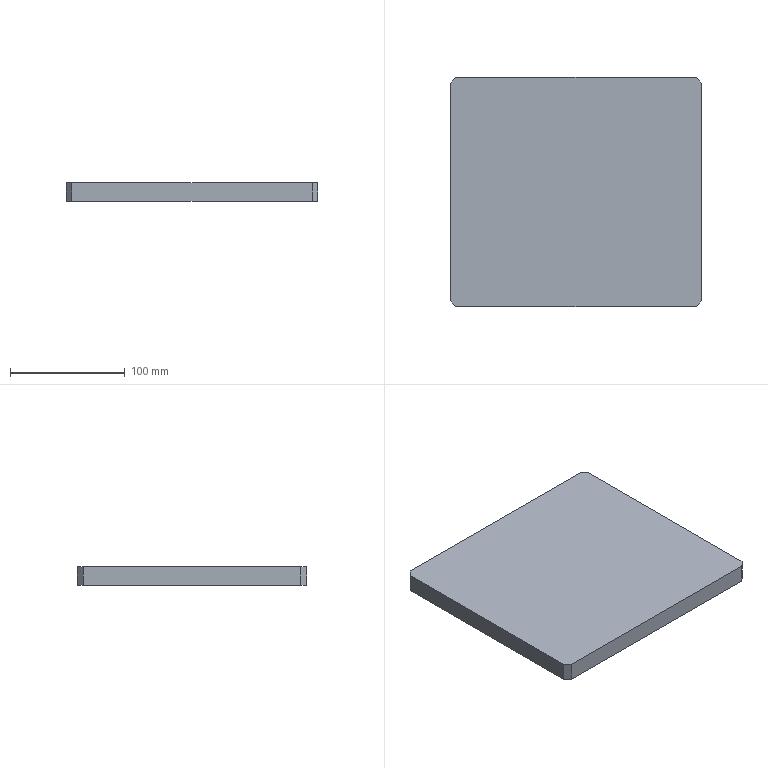Part | SolidWorks | features Chamfer 1, Extrusion 1 | 1 solid | 10 faces | box 220 x 200 x 16 mm | volume 703200 mm3 | plane 10
STEP:
#1=CARTESIAN_POINT('',(0.,-5.,0.));
#2=VERTEX_POINT('',#1);
#3=CARTESIAN_POINT('',(0.,-195.,0.));
#4=VERTEX_POINT('',#3);
#5=CARTESIAN_POINT('',(0.,0.,0.));
#6=DIRECTION('',(0.,-1.,0.));
#7=VECTOR('',#6,1000.);
#8=LINE('',#5,#7);
#9=EDGE_CURVE('',#2,#4,#8,.T.);
#10=ORIENTED_EDGE('',*,*,#9,.T.);
#11=CARTESIAN_POINT('',(0.,-195.,16.));
#12=VERTEX_POINT('',#11);
#13=CARTESIAN_POINT('',(0.,-195.,16.));
#14=DIRECTION('',(0.,0.,1.));
#15=VECTOR('',#14,1000.);
#16=LINE('',#13,#15);
#17=EDGE_CURVE('',#4,#12,#16,.T.);
#18=ORIENTED_EDGE('',*,*,#17,.T.);
#19=CARTESIAN_POINT('',(0.,-5.,16.));
#20=VERTEX_POINT('',#19);
#21=CARTESIAN_POINT('',(0.,0.,16.));
#22=DIRECTION('',(0.,-1.,0.));
#23=VECTOR('',#22,1000.);
#24=LINE('',#21,#23);
#25=EDGE_CURVE('',#20,#12,#24,.T.);
#26=ORIENTED_EDGE('',*,*,#25,.F.);
#27=CARTESIAN_POINT('',(0.,-5.,16.));
#28=DIRECTION('',(0.,0.,-1.));
#29=VECTOR('',#28,1000.);
#30=LINE('',#27,#29);
#31=EDGE_CURVE('',#20,#2,#30,.T.);
#32=ORIENTED_EDGE('',*,*,#31,.T.);
#33=EDGE_LOOP('',(#10,#18,#26,#32));
#34=FACE_OUTER_BOUND('',#33,.T.);
#35=CARTESIAN_POINT('',(0.,0.,16.));
#36=DIRECTION('',(1.,0.,0.));
#37=DIRECTION('',(0.,1.,0.));
#38=AXIS2_PLACEMENT_3D('',#35,#36,#37);
#39=PLANE('',#38);
#40=ADVANCED_FACE('',(#34),#39,.F.);
#41=CARTESIAN_POINT('',(5.,-200.,16.));
#42=VERTEX_POINT('',#41);
#43=CARTESIAN_POINT('',(215.,-200.,16.));
#44=VERTEX_POINT('',#43);
#45=CARTESIAN_POINT('',(0.,-200.,16.));
#46=DIRECTION('',(1.,0.,0.));
#47=VECTOR('',#46,1000.);
#48=LINE('',#45,#47);
#49=EDGE_CURVE('',#42,#44,#48,.T.);
#50=ORIENTED_EDGE('',*,*,#49,.F.);
#51=CARTESIAN_POINT('',(5.,-200.,0.));
#52=VERTEX_POINT('',#51);
#53=CARTESIAN_POINT('',(5.,-200.,16.));
#54=DIRECTION('',(0.,0.,-1.));
#55=VECTOR('',#54,1000.);
#56=LINE('',#53,#55);
#57=EDGE_CURVE('',#42,#52,#56,.T.);
#58=ORIENTED_EDGE('',*,*,#57,.T.);
#59=CARTESIAN_POINT('',(215.,-200.,0.));
#60=VERTEX_POINT('',#59);
#61=CARTESIAN_POINT('',(0.,-200.,0.));
#62=DIRECTION('',(1.,0.,0.));
#63=VECTOR('',#62,1000.);
#64=LINE('',#61,#63);
#65=EDGE_CURVE('',#52,#60,#64,.T.);
#66=ORIENTED_EDGE('',*,*,#65,.T.);
#67=CARTESIAN_POINT('',(215.,-200.,16.));
#68=DIRECTION('',(0.,0.,1.));
#69=VECTOR('',#68,1000.);
#70=LINE('',#67,#69);
#71=EDGE_CURVE('',#60,#44,#70,.T.);
#72=ORIENTED_EDGE('',*,*,#71,.T.);
#73=EDGE_LOOP('',(#50,#58,#66,#72));
#74=FACE_OUTER_BOUND('',#73,.T.);
#75=CARTESIAN_POINT('',(0.,-200.,16.));
#76=DIRECTION('',(0.,1.,0.));
#77=DIRECTION('',(0.,0.,1.));
#78=AXIS2_PLACEMENT_3D('',#75,#76,#77);
#79=PLANE('',#78);
#80=ADVANCED_FACE('',(#74),#79,.F.);
#81=CARTESIAN_POINT('',(220.,-195.,16.));
#82=VERTEX_POINT('',#81);
#83=CARTESIAN_POINT('',(220.,-5.,16.));
#84=VERTEX_POINT('',#83);
#85=CARTESIAN_POINT('',(220.,0.,16.));
#86=DIRECTION('',(0.,1.,0.));
#87=VECTOR('',#86,1000.);
#88=LINE('',#85,#87);
#89=EDGE_CURVE('',#82,#84,#88,.T.);
#90=ORIENTED_EDGE('',*,*,#89,.F.);
#91=CARTESIAN_POINT('',(220.,-195.,0.));
#92=VERTEX_POINT('',#91);
#93=CARTESIAN_POINT('',(220.,-195.,16.));
#94=DIRECTION('',(0.,0.,-1.));
#95=VECTOR('',#94,1000.);
#96=LINE('',#93,#95);
#97=EDGE_CURVE('',#82,#92,#96,.T.);
#98=ORIENTED_EDGE('',*,*,#97,.T.);
#99=CARTESIAN_POINT('',(220.,-5.,0.));
#100=VERTEX_POINT('',#99);
#101=CARTESIAN_POINT('',(220.,0.,0.));
#102=DIRECTION('',(0.,1.,0.));
#103=VECTOR('',#102,1000.);
#104=LINE('',#101,#103);
#105=EDGE_CURVE('',#92,#100,#104,.T.);
#106=ORIENTED_EDGE('',*,*,#105,.T.);
#107=CARTESIAN_POINT('',(220.,-5.,16.));
#108=DIRECTION('',(0.,0.,1.));
#109=VECTOR('',#108,1000.);
#110=LINE('',#107,#109);
#111=EDGE_CURVE('',#100,#84,#110,.T.);
#112=ORIENTED_EDGE('',*,*,#111,.T.);
#113=EDGE_LOOP('',(#90,#98,#106,#112));
#114=FACE_OUTER_BOUND('',#113,.T.);
#115=CARTESIAN_POINT('',(220.,0.,16.));
#116=DIRECTION('',(-1.,0.,0.));
#117=DIRECTION('',(0.,-1.,0.));
#118=AXIS2_PLACEMENT_3D('',#115,#116,#117);
#119=PLANE('',#118);
#120=ADVANCED_FACE('',(#114),#119,.F.);
#121=CARTESIAN_POINT('',(215.,0.,16.));
#122=VERTEX_POINT('',#121);
#123=CARTESIAN_POINT('',(5.,0.,16.));
#124=VERTEX_POINT('',#123);
#125=CARTESIAN_POINT('',(0.,0.,16.));
#126=DIRECTION('',(-1.,0.,0.));
#127=VECTOR('',#126,1000.);
#128=LINE('',#125,#127);
#129=EDGE_CURVE('',#122,#124,#128,.T.);
#130=ORIENTED_EDGE('',*,*,#129,.F.);
#131=CARTESIAN_POINT('',(215.,0.,0.));
#132=VERTEX_POINT('',#131);
#133=CARTESIAN_POINT('',(215.,0.,16.));
#134=DIRECTION('',(0.,0.,-1.));
#135=VECTOR('',#134,1000.);
#136=LINE('',#133,#135);
#137=EDGE_CURVE('',#122,#132,#136,.T.);
#138=ORIENTED_EDGE('',*,*,#137,.T.);
#139=CARTESIAN_POINT('',(5.,0.,0.));
#140=VERTEX_POINT('',#139);
#141=CARTESIAN_POINT('',(0.,0.,0.));
#142=DIRECTION('',(-1.,0.,0.));
#143=VECTOR('',#142,1000.);
#144=LINE('',#141,#143);
#145=EDGE_CURVE('',#132,#140,#144,.T.);
#146=ORIENTED_EDGE('',*,*,#145,.T.);
#147=CARTESIAN_POINT('',(5.,0.,16.));
#148=DIRECTION('',(0.,0.,1.));
#149=VECTOR('',#148,1000.);
#150=LINE('',#147,#149);
#151=EDGE_CURVE('',#140,#124,#150,.T.);
#152=ORIENTED_EDGE('',*,*,#151,.T.);
#153=EDGE_LOOP('',(#130,#138,#146,#152));
#154=FACE_OUTER_BOUND('',#153,.T.);
#155=CARTESIAN_POINT('',(0.,0.,16.));
#156=DIRECTION('',(0.,-1.,0.));
#157=DIRECTION('',(0.,0.,-1.));
#158=AXIS2_PLACEMENT_3D('',#155,#156,#157);
#159=PLANE('',#158);
#160=ADVANCED_FACE('',(#154),#159,.F.);
#161=ORIENTED_EDGE('',*,*,#25,.T.);
#162=CARTESIAN_POINT('',(-97.5,-97.5,16.));
#163=DIRECTION('',(0.7071,-0.7071,0.));
#164=VECTOR('',#163,1000.);
#165=LINE('',#162,#164);
#166=EDGE_CURVE('',#12,#42,#165,.T.);
#167=ORIENTED_EDGE('',*,*,#166,.T.);
#168=ORIENTED_EDGE('',*,*,#49,.T.);
#169=CARTESIAN_POINT('',(207.5,-207.5,16.));
#170=DIRECTION('',(0.7071,0.7071,0.));
#171=VECTOR('',#170,1000.);
#172=LINE('',#169,#171);
#173=EDGE_CURVE('',#44,#82,#172,.T.);
#174=ORIENTED_EDGE('',*,*,#173,.T.);
#175=ORIENTED_EDGE('',*,*,#89,.T.);
#176=CARTESIAN_POINT('',(107.5,107.5,16.));
#177=DIRECTION('',(-0.7071,0.7071,0.));
#178=VECTOR('',#177,1000.);
#179=LINE('',#176,#178);
#180=EDGE_CURVE('',#84,#122,#179,.T.);
#181=ORIENTED_EDGE('',*,*,#180,.T.);
#182=ORIENTED_EDGE('',*,*,#129,.T.);
#183=CARTESIAN_POINT('',(2.5,-2.5,16.));
#184=DIRECTION('',(-0.7071,-0.7071,0.));
#185=VECTOR('',#184,1000.);
#186=LINE('',#183,#185);
#187=EDGE_CURVE('',#124,#20,#186,.T.);
#188=ORIENTED_EDGE('',*,*,#187,.T.);
#189=EDGE_LOOP('',(#161,#167,#168,#174,#175,#181,#182,#188));
#190=FACE_OUTER_BOUND('',#189,.T.);
#191=CARTESIAN_POINT('',(0.,0.,16.));
#192=DIRECTION('',(0.,0.,1.));
#193=DIRECTION('',(1.,0.,0.));
#194=AXIS2_PLACEMENT_3D('',#191,#192,#193);
#195=PLANE('',#194);
#196=ADVANCED_FACE('',(#190),#195,.T.);
#197=ORIENTED_EDGE('',*,*,#65,.F.);
#198=CARTESIAN_POINT('',(5.,-200.,0.));
#199=DIRECTION('',(-0.7071,0.7071,0.));
#200=VECTOR('',#199,1000.);
#201=LINE('',#198,#200);
#202=EDGE_CURVE('',#52,#4,#201,.T.);
#203=ORIENTED_EDGE('',*,*,#202,.T.);
#204=ORIENTED_EDGE('',*,*,#9,.F.);
#205=CARTESIAN_POINT('',(0.,-5.,0.));
#206=DIRECTION('',(0.7071,0.7071,0.));
#207=VECTOR('',#206,1000.);
#208=LINE('',#205,#207);
#209=EDGE_CURVE('',#2,#140,#208,.T.);
#210=ORIENTED_EDGE('',*,*,#209,.T.);
#211=ORIENTED_EDGE('',*,*,#145,.F.);
#212=CARTESIAN_POINT('',(215.,0.,0.));
#213=DIRECTION('',(0.7071,-0.7071,0.));
#214=VECTOR('',#213,1000.);
#215=LINE('',#212,#214);
#216=EDGE_CURVE('',#132,#100,#215,.T.);
#217=ORIENTED_EDGE('',*,*,#216,.T.);
#218=ORIENTED_EDGE('',*,*,#105,.F.);
#219=CARTESIAN_POINT('',(220.,-195.,0.));
#220=DIRECTION('',(-0.7071,-0.7071,0.));
#221=VECTOR('',#220,1000.);
#222=LINE('',#219,#221);
#223=EDGE_CURVE('',#92,#60,#222,.T.);
#224=ORIENTED_EDGE('',*,*,#223,.T.);
#225=EDGE_LOOP('',(#197,#203,#204,#210,#211,#217,#218,#224));
#226=FACE_OUTER_BOUND('',#225,.T.);
#227=CARTESIAN_POINT('',(0.,0.,0.));
#228=DIRECTION('',(0.,0.,1.));
#229=DIRECTION('',(1.,0.,0.));
#230=AXIS2_PLACEMENT_3D('',#227,#228,#229);
#231=PLANE('',#230);
#232=ADVANCED_FACE('',(#226),#231,.F.);
#233=ORIENTED_EDGE('',*,*,#166,.F.);
#234=ORIENTED_EDGE('',*,*,#17,.F.);
#235=ORIENTED_EDGE('',*,*,#202,.F.);
#236=ORIENTED_EDGE('',*,*,#57,.F.);
#237=EDGE_LOOP('',(#233,#234,#235,#236));
#238=FACE_OUTER_BOUND('',#237,.T.);
#239=CARTESIAN_POINT('',(5.,-200.,16.));
#240=DIRECTION('',(0.7071,0.7071,0.));
#241=DIRECTION('',(0.,0.,-1.));
#242=AXIS2_PLACEMENT_3D('',#239,#240,#241);
#243=PLANE('',#242);
#244=ADVANCED_FACE('',(#238),#243,.F.);
#245=ORIENTED_EDGE('',*,*,#173,.F.);
#246=ORIENTED_EDGE('',*,*,#71,.F.);
#247=ORIENTED_EDGE('',*,*,#223,.F.);
#248=ORIENTED_EDGE('',*,*,#97,.F.);
#249=EDGE_LOOP('',(#245,#246,#247,#248));
#250=FACE_OUTER_BOUND('',#249,.T.);
#251=CARTESIAN_POINT('',(220.,-195.,16.));
#252=DIRECTION('',(-0.7071,0.7071,0.));
#253=DIRECTION('',(0.,0.,-1.));
#254=AXIS2_PLACEMENT_3D('',#251,#252,#253);
#255=PLANE('',#254);
#256=ADVANCED_FACE('',(#250),#255,.F.);
#257=ORIENTED_EDGE('',*,*,#180,.F.);
#258=ORIENTED_EDGE('',*,*,#111,.F.);
#259=ORIENTED_EDGE('',*,*,#216,.F.);
#260=ORIENTED_EDGE('',*,*,#137,.F.);
#261=EDGE_LOOP('',(#257,#258,#259,#260));
#262=FACE_OUTER_BOUND('',#261,.T.);
#263=CARTESIAN_POINT('',(215.,0.,16.));
#264=DIRECTION('',(-0.7071,-0.7071,0.));
#265=DIRECTION('',(0.,0.,-1.));
#266=AXIS2_PLACEMENT_3D('',#263,#264,#265);
#267=PLANE('',#266);
#268=ADVANCED_FACE('',(#262),#267,.F.);
#269=ORIENTED_EDGE('',*,*,#187,.F.);
#270=ORIENTED_EDGE('',*,*,#151,.F.);
#271=ORIENTED_EDGE('',*,*,#209,.F.);
#272=ORIENTED_EDGE('',*,*,#31,.F.);
#273=EDGE_LOOP('',(#269,#270,#271,#272));
#274=FACE_OUTER_BOUND('',#273,.T.);
#275=CARTESIAN_POINT('',(0.,-5.,16.));
#276=DIRECTION('',(0.7071,-0.7071,0.));
#277=DIRECTION('',(0.,0.,-1.));
#278=AXIS2_PLACEMENT_3D('',#275,#276,#277);
#279=PLANE('',#278);
#280=ADVANCED_FACE('',(#274),#279,.F.);
#281=CLOSED_SHELL('',(#40,#80,#120,#160,#196,#232,#244,#256,#268,#280));
#282=MANIFOLD_SOLID_BREP('',#281);
#283=CARTESIAN_POINT('',(0.,0.,0.));
#284=DIRECTION('',(0.,0.,1.));
#285=DIRECTION('',(1.,0.,0.));
#286=AXIS2_PLACEMENT_3D('',#283,#284,#285);
#287=(LENGTH_UNIT()NAMED_UNIT(*)SI_UNIT(.MILLI.,.METRE.));
#288=UNCERTAINTY_MEASURE_WITH_UNIT(LENGTH_MEASURE(0.00001),#287,'','');
#289=(NAMED_UNIT(*)PLANE_ANGLE_UNIT()SI_UNIT($,.RADIAN.));
#290=(NAMED_UNIT(*)SI_UNIT($,.STERADIAN.)SOLID_ANGLE_UNIT());
#291=(GEOMETRIC_REPRESENTATION_CONTEXT(3)GLOBAL_UNCERTAINTY_ASSIGNED_CONTEXT((#288))GLOBAL_UNIT_ASSIGNED_CONTEXT((#287,#289,#290))REPRESENTATION_CONTEXT('',''));
#292=ADVANCED_BREP_SHAPE_REPRESENTATION('',(#282,#286),#291);